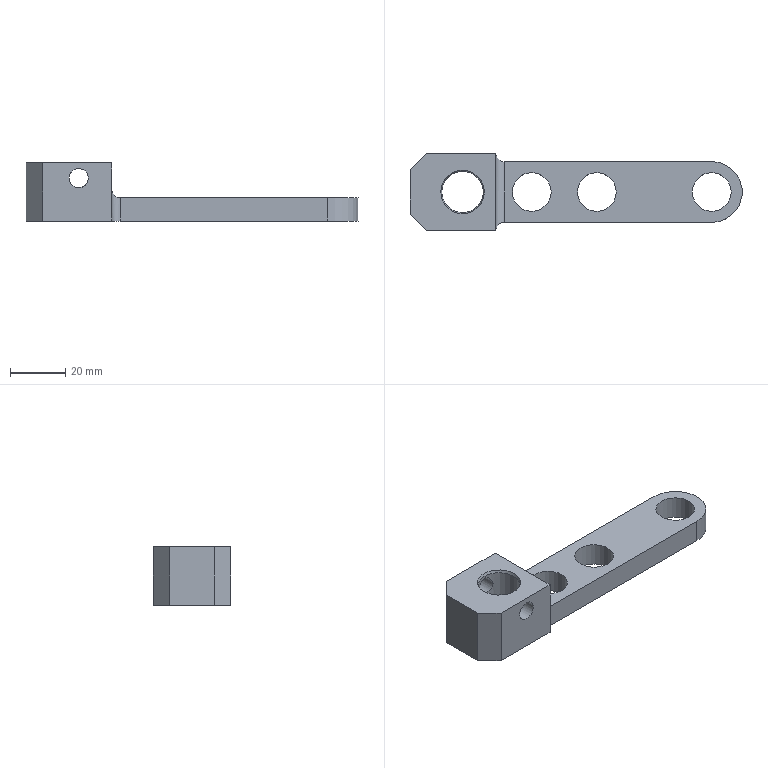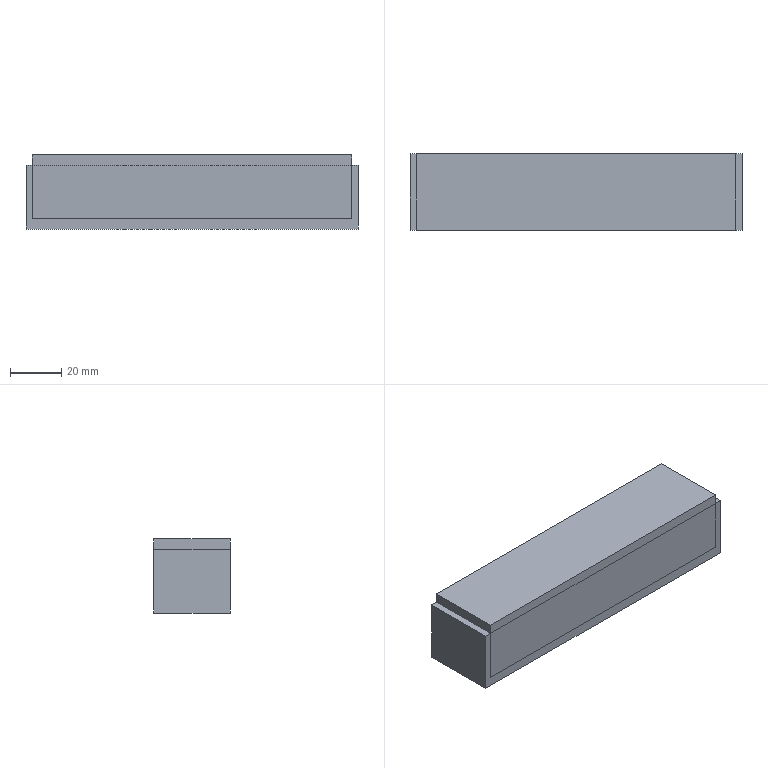CAM job | NX | 3+2 milling, drilling | part box 120 x 28 x 21 mm | stock box 130 x 30 x 29 mm
Tools:
number,name,description,diameter,corner_radius,flute_length,length,flutes
0,5R0.5,Milling Tool-5 Parameters,8.0,0.4,50.0,75.0,2
0,D5-15-D6-50-3T粗,D5-15-D6-50-3T,5.0,0.0,15.0,16.0,3
6,D6-18-D6-50-3T-精,D6-18-D6-50-3T,6.0,0.0,18.0,50.0,3
8,D8-25-D8-60-3T-精,D8-25-D8-60-3T,8.0,0.0,25.0,60.0,3
2,D10-30-D10-75-3T-粗,D10-30-D10-75-3T-粗,10.0,0.0,30.0,75.0,2
1,D50面刀,D50面刀,50.0,0.0,30.0,30.0,4
9,钻头D6.8-73-105,钻刀D6.8-73-105,6.8,0.0,73.0,105.0,2
4,钻头D13-114-152,钻刀D13-114-152,13.0,0.0,114.0,152.0,2
5,倒角D4-90度,倒角D4-90度,4.0,0.0,5.0,50.0,2
3,倒角D6-90度,倒角D6-90度,6.0,0.0,5.0,50.0,2
Operations:
program,operation,operation_type,tool,method,geometry_group,spindle_rpm,surface_speed,feed_per_tooth,feed_cut,feed_plunge,cut_length_mm,path_length_mm,cut_time_min,machine_time_min
A1,低壁铣光面,VolumeBased25DMillingOperation,D50面刀,METHOD,A-G54,3000.0,471.0,0.0667,800.0,100.0,181.971,215.971,0.2275,0.2309
A1,动态粗,CavityMilling,D10-30-D10-75-3T-粗,METHOD,WORKPIECE_54,4500.0,141.0,0.2222,2000.0,100.0,7308.307,7389.307,3.506,3.514
A1,DRILLING,Operation,倒角D6-90度,METHOD,WORKPIECE_54,1600.0,30.0,0.0187,60.0,0.0,16.0,171.478,0.2667,0.2822
A1,DRILLING_1,Operation,钻头D13-114-152,METHOD,WORKPIECE_54,800.0,32.0,0.0187,30.0,0.0,54.0,219.299,1.8,1.817
A1,DRILLING_1_COPY,Operation,钻头D13-114-152,METHOD,WORKPIECE_54,800.0,32.0,0.0187,30.0,0.0,30.0,100.0,1.0,1.007
A1,PLANAR_MILL,PlanarMilling,倒角D4-90度,METHOD,WORKPIECE_54,3000.0,37.0,0.1333,800.0,100.0,138.288,320.819,0.1729,0.1911
A1,PLANAR_MILL_COPY,PlanarMilling,倒角D4-90度,METHOD,WORKPIECE_54,3000.0,37.0,0.1333,800.0,100.0,296.661,335.661,0.3708,0.3747
A1,PLANAR_MILL_1_COPY,PlanarMilling,D6-18-D6-50-3T-精,METHOD,WORKPIECE_54,3000.0,56.0,0.0667,600.0,100.0,671.602,2828.67,1.119,1.335
A1,PLANAR_MILL_1,PlanarMilling,D6-18-D6-50-3T-精,METHOD,WORKPIECE_54,3000.0,56.0,0.0667,600.0,100.0,612.171,673.171,1.02,1.026
A1,PLANAR_MILL_1_COPY_1,PlanarMilling,D6-18-D6-50-3T-精,METHOD,WORKPIECE_54,3000.0,56.0,0.0667,600.0,100.0,212.791,402.791,0.3547,0.3737
A1,ZLEVEL_PROFILE_STEEP,ZLevelMilling,5R0.5,METHOD,WORKPIECE_54,4500.0,70.0,0.1111,1000.0,100.0,1346.644,1385.973,1.347,1.351
B1,动态粗_COPY,CavityMilling,D10-30-D10-75-3T-粗,METHOD,WORKPIECE_55,4500.0,141.0,0.2222,2000.0,100.0,23245.003,23484.245,11.431,11.455
B1,低壁铣光面_1,VolumeBased25DMillingOperation,D6-18-D6-50-3T-精,METHOD,WORKPIECE_55,4500.0,100.0,0.1178,700.0,100.0,937.455,1059.91,1.339,1.351
B1,ZLEVEL_PROFILE_STEEP_1,ZLevelMilling,5R0.5,METHOD,WORKPIECE_55,4500.0,70.0,0.2222,2000.0,100.0,6614.34,6637.289,3.307,3.309
B1,ZLEVEL_PROFILE_STEEP_COPY,ZLevelMilling,5R0.5,METHOD,WORKPIECE_55,4500.0,70.0,0.1111,1000.0,100.0,1366.282,1377.58,1.366,1.367
B1,PLANAR_MILL_3,PlanarMilling,倒角D4-90度,METHOD,WORKPIECE_55,3500.0,43.0,0.1143,800.0,100.0,130.679,141.679,0.1633,0.1644
B1,PLANAR_MILL_3_COPY_1,PlanarMilling,倒角D4-90度,METHOD,WORKPIECE_55,3500.0,43.0,0.1143,800.0,100.0,193.553,229.553,0.2419,0.2455
B1,PLANAR_MILL_3_COPY,PlanarMilling,倒角D4-90度,METHOD,WORKPIECE_55,3500.0,43.0,0.1143,800.0,100.0,138.288,311.819,0.1729,0.1902
B1,HOLE_MILLING,CylinderMilling,D8-25-D8-60-3T-精,METHOD,B-G55,3000.0,94.0,0.1333,800.0,100.0,2307.948,2501.948,2.885,2.904
B1,HOLE_MILLING_1,CylinderMilling,D8-25-D8-60-3T-精,METHOD,B-G55,3000.0,94.0,0.1333,800.0,100.0,1802.973,1833.473,2.254,2.257
B1,PLANAR_MILL_4,PlanarMilling,D8-25-D8-60-3T-精,METHOD,B-G55,3000.0,56.0,0.0222,200.0,100.0,99.719,150.719,0.4986,0.5037
B1,PLANAR_MILL_4_COPY,PlanarMilling,D8-25-D8-60-3T-精,METHOD,B-G55,3000.0,56.0,0.0222,200.0,100.0,271.594,489.701,1.358,1.38
C1,DRILLING_3,Operation,倒角D6-90度,METHOD,C-G56,1200.0,22.0,0.025,60.0,0.0,4.0,48.0,0.0667,0.0711
C1,DRILLING_4,Operation,钻头D6.8-73-105,METHOD,C-G56,800.0,17.0,0.0375,60.0,0.0,13.0,66.0,0.2167,0.222
C1,PLANAR_MILL_5_COPY_COPY,PlanarMilling,倒角D6-90度,METHOD,C-G56,3000.0,56.0,0.01,60.0,100.0,15.466,55.466,0.2578,0.2618
C1,PLANAR_MILL_5,PlanarMilling,D6-18-D6-50-3T-精,METHOD,C-G56,3000.0,56.0,0.0067,60.0,100.0,20.338,74.338,0.339,0.3444
C1,PLANAR_MILL_5_COPY,PlanarMilling,D6-18-D6-50-3T-精,METHOD,C-G56,3000.0,56.0,0.0033,30.0,100.0,18.834,72.834,0.6278,0.6332
D1,DRILLING_3_COPY,Operation,倒角D6-90度,METHOD,WORKPIECE_57,1200.0,22.0,0.025,60.0,0.0,4.0,48.0,0.0667,0.0711
D1,DRILLING_4_COPY,Operation,钻头D6.8-73-105,METHOD,WORKPIECE_57,800.0,17.0,0.0375,60.0,0.0,13.0,66.0,0.2167,0.222
D1,PLANAR_MILL_5_COPY_COPY_COPY,PlanarMilling,倒角D6-90度,METHOD,WORKPIECE_57,3000.0,56.0,0.01,60.0,100.0,15.466,55.466,0.2578,0.2618
D1,PLANAR_MILL_5_COPY_1,PlanarMilling,D6-18-D6-50-3T-精,METHOD,WORKPIECE_57,3000.0,56.0,0.0067,60.0,100.0,20.338,74.338,0.339,0.3444
D1,PLANAR_MILL_5_COPY_COPY_1,PlanarMilling,D6-18-D6-50-3T-精,METHOD,WORKPIECE_57,3000.0,56.0,0.0033,30.0,100.0,18.834,72.834,0.6278,0.6332
工装1,PLANAR_MILL_2,PlanarMilling,D5-15-D6-50-3T粗,METHOD,GZ1,4500.0,84.0,0.0889,800.0,100.0,5946.371,6296.719,7.433,7.468
工装1,DRILLING_2,Operation,D5-15-D6-50-3T粗,METHOD,GZ1,2000.0,31.0,0.0333,200.0,0.0,63.0,228.637,0.315,0.3316
工装1,PLANAR_MILL_2_COPY,PlanarMilling,D5-15-D6-50-3T粗,METHOD,GZ1,4500.0,84.0,0.0889,800.0,100.0,1016.043,1063.043,1.27,1.275
工装1,PLANAR_MILL_2_COPY_COPY,PlanarMilling,D5-15-D6-50-3T粗,METHOD,GZ1,4500.0,84.0,0.0889,800.0,100.0,271.963,320.963,0.34,0.3449